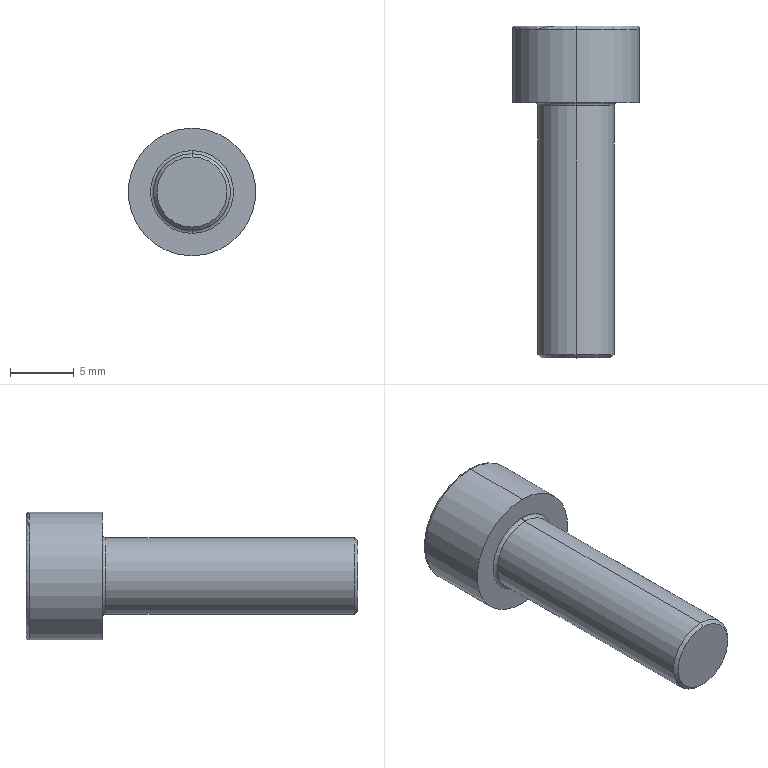Part | STEP file | 1 solid | 20 faces | box 10 x 26 x 10 mm | volume 971.042 mm3 | plane 10 | torus 4 | cylinder 4 | cone 2 | commonest cylinder face diameters 6 x2 10 x2
STEP:
#1=CARTESIAN_POINT('',(0.,-20.,-2.75));
#2=VERTEX_POINT('',#1);
#3=CARTESIAN_POINT('',(0.,-20.,2.75));
#4=VERTEX_POINT('',#3);
#5=CARTESIAN_POINT('',(0.,-20.,0.));
#6=DIRECTION('',(0.,-1.,0.));
#7=DIRECTION('',(0.,0.,-1.));
#8=AXIS2_PLACEMENT_3D('',#5,#6,#7);
#9=CIRCLE('',#8,2.75);
#10=EDGE_CURVE('',#2,#4,#9,.T.);
#11=ORIENTED_EDGE('',*,*,#10,.F.);
#12=CARTESIAN_POINT('',(0.,-19.75,-3.));
#13=VERTEX_POINT('',#12);
#14=CARTESIAN_POINT('',(0.,-20.,-2.75));
#15=DIRECTION('',(0.,0.7071,-0.7071));
#16=VECTOR('',#15,1000.);
#17=LINE('',#14,#16);
#18=EDGE_CURVE('',#2,#13,#17,.T.);
#19=ORIENTED_EDGE('',*,*,#18,.T.);
#20=CARTESIAN_POINT('',(0.,-19.75,3.));
#21=VERTEX_POINT('',#20);
#22=CARTESIAN_POINT('',(0.,-19.75,0.));
#23=DIRECTION('',(0.,1.,0.));
#24=DIRECTION('',(0.,0.,-1.));
#25=AXIS2_PLACEMENT_3D('',#22,#23,#24);
#26=CIRCLE('',#25,3.);
#27=EDGE_CURVE('',#21,#13,#26,.T.);
#28=ORIENTED_EDGE('',*,*,#27,.F.);
#29=CARTESIAN_POINT('',(0.,-20.,2.75));
#30=DIRECTION('',(0.,0.7071,0.7071));
#31=VECTOR('',#30,1000.);
#32=LINE('',#29,#31);
#33=EDGE_CURVE('',#4,#21,#32,.T.);
#34=ORIENTED_EDGE('',*,*,#33,.F.);
#35=EDGE_LOOP('',(#11,#19,#28,#34));
#36=FACE_OUTER_BOUND('',#35,.T.);
#37=CARTESIAN_POINT('',(0.,-20.,0.));
#38=DIRECTION('',(0.,1.,0.));
#39=DIRECTION('',(0.,0.,1.));
#40=AXIS2_PLACEMENT_3D('',#37,#38,#39);
#41=CONICAL_SURFACE('',#40,2.75,0.7854);
#42=ADVANCED_FACE('',(#36),#41,.T.);
#43=CARTESIAN_POINT('',(0.,5.75,-5.));
#44=VERTEX_POINT('',#43);
#45=CARTESIAN_POINT('',(0.,5.75,5.));
#46=VERTEX_POINT('',#45);
#47=CARTESIAN_POINT('',(0.,5.75,0.));
#48=DIRECTION('',(0.,-1.,0.));
#49=DIRECTION('',(0.,0.,1.));
#50=AXIS2_PLACEMENT_3D('',#47,#48,#49);
#51=CIRCLE('',#50,5.);
#52=EDGE_CURVE('',#44,#46,#51,.T.);
#53=ORIENTED_EDGE('',*,*,#52,.F.);
#54=CARTESIAN_POINT('',(0.,6.,-4.75));
#55=VERTEX_POINT('',#54);
#56=CARTESIAN_POINT('',(0.,5.75,-4.75));
#57=DIRECTION('',(1.,0.,0.));
#58=DIRECTION('',(0.,0.,-1.));
#59=AXIS2_PLACEMENT_3D('',#56,#57,#58);
#60=CIRCLE('',#59,0.25);
#61=EDGE_CURVE('',#44,#55,#60,.T.);
#62=ORIENTED_EDGE('',*,*,#61,.T.);
#63=CARTESIAN_POINT('',(0.,6.,4.75));
#64=VERTEX_POINT('',#63);
#65=CARTESIAN_POINT('',(0.,6.,0.));
#66=DIRECTION('',(0.,1.,0.));
#67=DIRECTION('',(0.,0.,1.));
#68=AXIS2_PLACEMENT_3D('',#65,#66,#67);
#69=CIRCLE('',#68,4.75);
#70=EDGE_CURVE('',#64,#55,#69,.T.);
#71=ORIENTED_EDGE('',*,*,#70,.F.);
#72=CARTESIAN_POINT('',(0.,5.75,4.75));
#73=DIRECTION('',(-1.,0.,0.));
#74=DIRECTION('',(0.,0.,1.));
#75=AXIS2_PLACEMENT_3D('',#72,#73,#74);
#76=CIRCLE('',#75,0.25);
#77=EDGE_CURVE('',#46,#64,#76,.T.);
#78=ORIENTED_EDGE('',*,*,#77,.F.);
#79=EDGE_LOOP('',(#53,#62,#71,#78));
#80=FACE_OUTER_BOUND('',#79,.T.);
#81=CARTESIAN_POINT('',(0.,5.75,0.));
#82=DIRECTION('',(0.,1.,0.));
#83=DIRECTION('',(0.,0.,1.));
#84=AXIS2_PLACEMENT_3D('',#81,#82,#83);
#85=TOROIDAL_SURFACE('',#84,4.75,0.25);
#86=ADVANCED_FACE('',(#80),#85,.T.);
#87=CARTESIAN_POINT('',(0.,-0.25,3.));
#88=VERTEX_POINT('',#87);
#89=CARTESIAN_POINT('',(0.,-0.25,-3.));
#90=VERTEX_POINT('',#89);
#91=CARTESIAN_POINT('',(0.,-0.25,0.));
#92=DIRECTION('',(0.,-1.,0.));
#93=DIRECTION('',(0.,0.,-1.));
#94=AXIS2_PLACEMENT_3D('',#91,#92,#93);
#95=CIRCLE('',#94,3.);
#96=EDGE_CURVE('',#88,#90,#95,.T.);
#97=ORIENTED_EDGE('',*,*,#96,.F.);
#98=CARTESIAN_POINT('',(0.,0.,3.25));
#99=VERTEX_POINT('',#98);
#100=CARTESIAN_POINT('',(0.,-0.25,3.25));
#101=DIRECTION('',(1.,0.,0.));
#102=DIRECTION('',(0.,0.,-1.));
#103=AXIS2_PLACEMENT_3D('',#100,#101,#102);
#104=CIRCLE('',#103,0.25);
#105=EDGE_CURVE('',#88,#99,#104,.T.);
#106=ORIENTED_EDGE('',*,*,#105,.T.);
#107=CARTESIAN_POINT('',(0.,0.,-3.25));
#108=VERTEX_POINT('',#107);
#109=CARTESIAN_POINT('',(0.,0.,0.));
#110=DIRECTION('',(0.,1.,0.));
#111=DIRECTION('',(0.,0.,-1.));
#112=AXIS2_PLACEMENT_3D('',#109,#110,#111);
#113=CIRCLE('',#112,3.25);
#114=EDGE_CURVE('',#108,#99,#113,.T.);
#115=ORIENTED_EDGE('',*,*,#114,.F.);
#116=CARTESIAN_POINT('',(0.,-0.25,-3.25));
#117=DIRECTION('',(-1.,0.,0.));
#118=DIRECTION('',(0.,0.,1.));
#119=AXIS2_PLACEMENT_3D('',#116,#117,#118);
#120=CIRCLE('',#119,0.25);
#121=EDGE_CURVE('',#90,#108,#120,.T.);
#122=ORIENTED_EDGE('',*,*,#121,.F.);
#123=EDGE_LOOP('',(#97,#106,#115,#122));
#124=FACE_OUTER_BOUND('',#123,.T.);
#125=CARTESIAN_POINT('',(0.,-0.25,0.));
#126=DIRECTION('',(0.,-1.,0.));
#127=DIRECTION('',(0.,0.,-1.));
#128=AXIS2_PLACEMENT_3D('',#125,#126,#127);
#129=TOROIDAL_SURFACE('',#128,3.25,0.25);
#130=ADVANCED_FACE('',(#124),#129,.F.);
#131=CARTESIAN_POINT('',(0.,-0.25,0.));
#132=DIRECTION('',(0.,-1.,0.));
#133=DIRECTION('',(0.,0.,-1.));
#134=AXIS2_PLACEMENT_3D('',#131,#132,#133);
#135=CIRCLE('',#134,3.);
#136=EDGE_CURVE('',#90,#88,#135,.T.);
#137=ORIENTED_EDGE('',*,*,#136,.T.);
#138=CARTESIAN_POINT('',(0.,0.,3.));
#139=DIRECTION('',(0.,-1.,0.));
#140=VECTOR('',#139,1000.);
#141=LINE('',#138,#140);
#142=EDGE_CURVE('',#88,#21,#141,.T.);
#143=ORIENTED_EDGE('',*,*,#142,.T.);
#144=ORIENTED_EDGE('',*,*,#27,.T.);
#145=CARTESIAN_POINT('',(0.,0.,-3.));
#146=DIRECTION('',(0.,-1.,0.));
#147=VECTOR('',#146,1000.);
#148=LINE('',#145,#147);
#149=EDGE_CURVE('',#90,#13,#148,.T.);
#150=ORIENTED_EDGE('',*,*,#149,.F.);
#151=EDGE_LOOP('',(#137,#143,#144,#150));
#152=FACE_OUTER_BOUND('',#151,.T.);
#153=CARTESIAN_POINT('',(0.,0.,0.));
#154=DIRECTION('',(0.,-1.,0.));
#155=DIRECTION('',(0.,0.,-1.));
#156=AXIS2_PLACEMENT_3D('',#153,#154,#155);
#157=CYLINDRICAL_SURFACE('',#156,3.);
#158=ADVANCED_FACE('',(#152),#157,.T.);
#159=ORIENTED_EDGE('',*,*,#52,.T.);
#160=CARTESIAN_POINT('',(0.,0.,5.));
#161=VERTEX_POINT('',#160);
#162=CARTESIAN_POINT('',(0.,0.,5.));
#163=DIRECTION('',(0.,-1.,0.));
#164=VECTOR('',#163,1000.);
#165=LINE('',#162,#164);
#166=EDGE_CURVE('',#46,#161,#165,.T.);
#167=ORIENTED_EDGE('',*,*,#166,.T.);
#168=CARTESIAN_POINT('',(0.,0.,-5.));
#169=VERTEX_POINT('',#168);
#170=CARTESIAN_POINT('',(0.,0.,0.));
#171=DIRECTION('',(0.,-1.,0.));
#172=DIRECTION('',(0.,0.,-1.));
#173=AXIS2_PLACEMENT_3D('',#170,#171,#172);
#174=CIRCLE('',#173,5.);
#175=EDGE_CURVE('',#169,#161,#174,.T.);
#176=ORIENTED_EDGE('',*,*,#175,.F.);
#177=CARTESIAN_POINT('',(0.,0.,-5.));
#178=DIRECTION('',(0.,-1.,0.));
#179=VECTOR('',#178,1000.);
#180=LINE('',#177,#179);
#181=EDGE_CURVE('',#44,#169,#180,.T.);
#182=ORIENTED_EDGE('',*,*,#181,.F.);
#183=EDGE_LOOP('',(#159,#167,#176,#182));
#184=FACE_OUTER_BOUND('',#183,.T.);
#185=CARTESIAN_POINT('',(0.,0.,0.));
#186=DIRECTION('',(0.,-1.,0.));
#187=DIRECTION('',(0.,0.,-1.));
#188=AXIS2_PLACEMENT_3D('',#185,#186,#187);
#189=CYLINDRICAL_SURFACE('',#188,5.);
#190=ADVANCED_FACE('',(#184),#189,.T.);
#191=ORIENTED_EDGE('',*,*,#70,.T.);
#192=CARTESIAN_POINT('',(0.,6.,0.));
#193=DIRECTION('',(0.,1.,0.));
#194=DIRECTION('',(0.,0.,1.));
#195=AXIS2_PLACEMENT_3D('',#192,#193,#194);
#196=CIRCLE('',#195,4.75);
#197=EDGE_CURVE('',#55,#64,#196,.T.);
#198=ORIENTED_EDGE('',*,*,#197,.T.);
#199=EDGE_LOOP('',(#191,#198));
#200=FACE_OUTER_BOUND('',#199,.T.);
#201=CARTESIAN_POINT('',(0.,6.,-2.887));
#202=VERTEX_POINT('',#201);
#203=CARTESIAN_POINT('',(-2.5,6.,-1.443));
#204=VERTEX_POINT('',#203);
#205=CARTESIAN_POINT('',(0.,6.,-2.887));
#206=DIRECTION('',(-0.866,0.,0.5));
#207=VECTOR('',#206,1000.);
#208=LINE('',#205,#207);
#209=EDGE_CURVE('',#202,#204,#208,.T.);
#210=ORIENTED_EDGE('',*,*,#209,.F.);
#211=CARTESIAN_POINT('',(2.5,6.,-1.443));
#212=VERTEX_POINT('',#211);
#213=CARTESIAN_POINT('',(2.5,6.,-1.443));
#214=DIRECTION('',(-0.866,0.,-0.5));
#215=VECTOR('',#214,1000.);
#216=LINE('',#213,#215);
#217=EDGE_CURVE('',#212,#202,#216,.T.);
#218=ORIENTED_EDGE('',*,*,#217,.F.);
#219=CARTESIAN_POINT('',(2.5,6.,1.443));
#220=VERTEX_POINT('',#219);
#221=CARTESIAN_POINT('',(2.5,6.,1.443));
#222=DIRECTION('',(0.,0.,-1.));
#223=VECTOR('',#222,1000.);
#224=LINE('',#221,#223);
#225=EDGE_CURVE('',#220,#212,#224,.T.);
#226=ORIENTED_EDGE('',*,*,#225,.F.);
#227=CARTESIAN_POINT('',(0.,6.,2.887));
#228=VERTEX_POINT('',#227);
#229=CARTESIAN_POINT('',(0.,6.,2.887));
#230=DIRECTION('',(0.866,0.,-0.5));
#231=VECTOR('',#230,1000.);
#232=LINE('',#229,#231);
#233=EDGE_CURVE('',#228,#220,#232,.T.);
#234=ORIENTED_EDGE('',*,*,#233,.F.);
#235=CARTESIAN_POINT('',(-2.5,6.,1.443));
#236=VERTEX_POINT('',#235);
#237=CARTESIAN_POINT('',(-2.5,6.,1.443));
#238=DIRECTION('',(0.866,0.,0.5));
#239=VECTOR('',#238,1000.);
#240=LINE('',#237,#239);
#241=EDGE_CURVE('',#236,#228,#240,.T.);
#242=ORIENTED_EDGE('',*,*,#241,.F.);
#243=CARTESIAN_POINT('',(-2.5,6.,-1.443));
#244=DIRECTION('',(0.,0.,1.));
#245=VECTOR('',#244,1000.);
#246=LINE('',#243,#245);
#247=EDGE_CURVE('',#204,#236,#246,.T.);
#248=ORIENTED_EDGE('',*,*,#247,.F.);
#249=EDGE_LOOP('',(#210,#218,#226,#234,#242,#248));
#250=FACE_BOUND('',#249,.T.);
#251=CARTESIAN_POINT('',(0.,6.,0.));
#252=DIRECTION('',(0.,1.,0.));
#253=DIRECTION('',(0.,0.,1.));
#254=AXIS2_PLACEMENT_3D('',#251,#252,#253);
#255=PLANE('',#254);
#256=ADVANCED_FACE('',(#200,#250),#255,.T.);
#257=ORIENTED_EDGE('',*,*,#166,.F.);
#258=CARTESIAN_POINT('',(0.,5.75,0.));
#259=DIRECTION('',(0.,-1.,0.));
#260=DIRECTION('',(0.,0.,1.));
#261=AXIS2_PLACEMENT_3D('',#258,#259,#260);
#262=CIRCLE('',#261,5.);
#263=EDGE_CURVE('',#46,#44,#262,.T.);
#264=ORIENTED_EDGE('',*,*,#263,.T.);
#265=ORIENTED_EDGE('',*,*,#181,.T.);
#266=CARTESIAN_POINT('',(0.,0.,0.));
#267=DIRECTION('',(0.,-1.,0.));
#268=DIRECTION('',(0.,0.,-1.));
#269=AXIS2_PLACEMENT_3D('',#266,#267,#268);
#270=CIRCLE('',#269,5.);
#271=EDGE_CURVE('',#161,#169,#270,.T.);
#272=ORIENTED_EDGE('',*,*,#271,.F.);
#273=EDGE_LOOP('',(#257,#264,#265,#272));
#274=FACE_OUTER_BOUND('',#273,.T.);
#275=CARTESIAN_POINT('',(0.,0.,0.));
#276=DIRECTION('',(0.,-1.,0.));
#277=DIRECTION('',(0.,0.,-1.));
#278=AXIS2_PLACEMENT_3D('',#275,#276,#277);
#279=CYLINDRICAL_SURFACE('',#278,5.);
#280=ADVANCED_FACE('',(#274),#279,.T.);
#281=ORIENTED_EDGE('',*,*,#114,.T.);
#282=CARTESIAN_POINT('',(0.,0.,0.));
#283=DIRECTION('',(0.,1.,0.));
#284=DIRECTION('',(0.,0.,-1.));
#285=AXIS2_PLACEMENT_3D('',#282,#283,#284);
#286=CIRCLE('',#285,3.25);
#287=EDGE_CURVE('',#99,#108,#286,.T.);
#288=ORIENTED_EDGE('',*,*,#287,.T.);
#289=EDGE_LOOP('',(#281,#288));
#290=FACE_BOUND('',#289,.T.);
#291=ORIENTED_EDGE('',*,*,#175,.T.);
#292=ORIENTED_EDGE('',*,*,#271,.T.);
#293=EDGE_LOOP('',(#291,#292));
#294=FACE_OUTER_BOUND('',#293,.T.);
#295=CARTESIAN_POINT('',(5.,0.,0.));
#296=DIRECTION('',(0.,-1.,0.));
#297=DIRECTION('',(0.,0.,-1.));
#298=AXIS2_PLACEMENT_3D('',#295,#296,#297);
#299=PLANE('',#298);
#300=ADVANCED_FACE('',(#290,#294),#299,.T.);
#301=ORIENTED_EDGE('',*,*,#142,.F.);
#302=ORIENTED_EDGE('',*,*,#96,.T.);
#303=ORIENTED_EDGE('',*,*,#149,.T.);
#304=CARTESIAN_POINT('',(0.,-19.75,0.));
#305=DIRECTION('',(0.,1.,0.));
#306=DIRECTION('',(0.,0.,-1.));
#307=AXIS2_PLACEMENT_3D('',#304,#305,#306);
#308=CIRCLE('',#307,3.);
#309=EDGE_CURVE('',#13,#21,#308,.T.);
#310=ORIENTED_EDGE('',*,*,#309,.T.);
#311=EDGE_LOOP('',(#301,#302,#303,#310));
#312=FACE_OUTER_BOUND('',#311,.T.);
#313=CARTESIAN_POINT('',(0.,0.,0.));
#314=DIRECTION('',(0.,-1.,0.));
#315=DIRECTION('',(0.,0.,-1.));
#316=AXIS2_PLACEMENT_3D('',#313,#314,#315);
#317=CYLINDRICAL_SURFACE('',#316,3.);
#318=ADVANCED_FACE('',(#312),#317,.T.);
#319=CARTESIAN_POINT('',(0.,-20.,0.));
#320=DIRECTION('',(0.,-1.,0.));
#321=DIRECTION('',(0.,0.,-1.));
#322=AXIS2_PLACEMENT_3D('',#319,#320,#321);
#323=CIRCLE('',#322,2.75);
#324=EDGE_CURVE('',#4,#2,#323,.T.);
#325=ORIENTED_EDGE('',*,*,#324,.T.);
#326=ORIENTED_EDGE('',*,*,#10,.T.);
#327=EDGE_LOOP('',(#325,#326));
#328=FACE_OUTER_BOUND('',#327,.T.);
#329=CARTESIAN_POINT('',(3.,-20.,0.));
#330=DIRECTION('',(0.,-1.,0.));
#331=DIRECTION('',(0.,0.,-1.));
#332=AXIS2_PLACEMENT_3D('',#329,#330,#331);
#333=PLANE('',#332);
#334=ADVANCED_FACE('',(#328),#333,.T.);
#335=ORIENTED_EDGE('',*,*,#209,.T.);
#336=CARTESIAN_POINT('',(-2.5,3.,-1.443));
#337=VERTEX_POINT('',#336);
#338=CARTESIAN_POINT('',(-2.5,3.,-1.443));
#339=DIRECTION('',(0.,1.,0.));
#340=VECTOR('',#339,1000.);
#341=LINE('',#338,#340);
#342=EDGE_CURVE('',#337,#204,#341,.T.);
#343=ORIENTED_EDGE('',*,*,#342,.F.);
#344=CARTESIAN_POINT('',(0.,3.,-2.887));
#345=VERTEX_POINT('',#344);
#346=CARTESIAN_POINT('',(0.,3.,-2.887));
#347=DIRECTION('',(-0.866,0.,0.5));
#348=VECTOR('',#347,1000.);
#349=LINE('',#346,#348);
#350=EDGE_CURVE('',#345,#337,#349,.T.);
#351=ORIENTED_EDGE('',*,*,#350,.F.);
#352=CARTESIAN_POINT('',(0.,3.,-2.887));
#353=DIRECTION('',(0.,1.,0.));
#354=VECTOR('',#353,1000.);
#355=LINE('',#352,#354);
#356=EDGE_CURVE('',#345,#202,#355,.T.);
#357=ORIENTED_EDGE('',*,*,#356,.T.);
#358=EDGE_LOOP('',(#335,#343,#351,#357));
#359=FACE_OUTER_BOUND('',#358,.T.);
#360=CARTESIAN_POINT('',(0.,3.,-2.887));
#361=DIRECTION('',(-0.5,0.,-0.866));
#362=DIRECTION('',(-0.866,0.,0.5));
#363=AXIS2_PLACEMENT_3D('',#360,#361,#362);
#364=PLANE('',#363);
#365=ADVANCED_FACE('',(#359),#364,.F.);
#366=ORIENTED_EDGE('',*,*,#217,.T.);
#367=ORIENTED_EDGE('',*,*,#356,.F.);
#368=CARTESIAN_POINT('',(2.5,3.,-1.443));
#369=VERTEX_POINT('',#368);
#370=CARTESIAN_POINT('',(2.5,3.,-1.443));
#371=DIRECTION('',(-0.866,0.,-0.5));
#372=VECTOR('',#371,1000.);
#373=LINE('',#370,#372);
#374=EDGE_CURVE('',#369,#345,#373,.T.);
#375=ORIENTED_EDGE('',*,*,#374,.F.);
#376=CARTESIAN_POINT('',(2.5,3.,-1.443));
#377=DIRECTION('',(0.,1.,0.));
#378=VECTOR('',#377,1000.);
#379=LINE('',#376,#378);
#380=EDGE_CURVE('',#369,#212,#379,.T.);
#381=ORIENTED_EDGE('',*,*,#380,.T.);
#382=EDGE_LOOP('',(#366,#367,#375,#381));
#383=FACE_OUTER_BOUND('',#382,.T.);
#384=CARTESIAN_POINT('',(2.5,3.,-1.443));
#385=DIRECTION('',(0.5,0.,-0.866));
#386=DIRECTION('',(-0.866,0.,-0.5));
#387=AXIS2_PLACEMENT_3D('',#384,#385,#386);
#388=PLANE('',#387);
#389=ADVANCED_FACE('',(#383),#388,.F.);
#390=ORIENTED_EDGE('',*,*,#225,.T.);
#391=ORIENTED_EDGE('',*,*,#380,.F.);
#392=CARTESIAN_POINT('',(2.5,3.,1.443));
#393=VERTEX_POINT('',#392);
#394=CARTESIAN_POINT('',(2.5,3.,1.443));
#395=DIRECTION('',(0.,0.,-1.));
#396=VECTOR('',#395,1000.);
#397=LINE('',#394,#396);
#398=EDGE_CURVE('',#393,#369,#397,.T.);
#399=ORIENTED_EDGE('',*,*,#398,.F.);
#400=CARTESIAN_POINT('',(2.5,3.,1.443));
#401=DIRECTION('',(0.,1.,0.));
#402=VECTOR('',#401,1000.);
#403=LINE('',#400,#402);
#404=EDGE_CURVE('',#393,#220,#403,.T.);
#405=ORIENTED_EDGE('',*,*,#404,.T.);
#406=EDGE_LOOP('',(#390,#391,#399,#405));
#407=FACE_OUTER_BOUND('',#406,.T.);
#408=CARTESIAN_POINT('',(2.5,3.,1.443));
#409=DIRECTION('',(1.,0.,0.));
#410=DIRECTION('',(0.,0.,-1.));
#411=AXIS2_PLACEMENT_3D('',#408,#409,#410);
#412=PLANE('',#411);
#413=ADVANCED_FACE('',(#407),#412,.F.);
#414=ORIENTED_EDGE('',*,*,#233,.T.);
#415=ORIENTED_EDGE('',*,*,#404,.F.);
#416=CARTESIAN_POINT('',(0.,3.,2.887));
#417=VERTEX_POINT('',#416);
#418=CARTESIAN_POINT('',(0.,3.,2.887));
#419=DIRECTION('',(0.866,0.,-0.5));
#420=VECTOR('',#419,1000.);
#421=LINE('',#418,#420);
#422=EDGE_CURVE('',#417,#393,#421,.T.);
#423=ORIENTED_EDGE('',*,*,#422,.F.);
#424=CARTESIAN_POINT('',(0.,3.,2.887));
#425=DIRECTION('',(0.,1.,0.));
#426=VECTOR('',#425,1000.);
#427=LINE('',#424,#426);
#428=EDGE_CURVE('',#417,#228,#427,.T.);
#429=ORIENTED_EDGE('',*,*,#428,.T.);
#430=EDGE_LOOP('',(#414,#415,#423,#429));
#431=FACE_OUTER_BOUND('',#430,.T.);
#432=CARTESIAN_POINT('',(0.,3.,2.887));
#433=DIRECTION('',(0.5,0.,0.866));
#434=DIRECTION('',(0.866,0.,-0.5));
#435=AXIS2_PLACEMENT_3D('',#432,#433,#434);
#436=PLANE('',#435);
#437=ADVANCED_FACE('',(#431),#436,.F.);
#438=ORIENTED_EDGE('',*,*,#241,.T.);
#439=ORIENTED_EDGE('',*,*,#428,.F.);
#440=CARTESIAN_POINT('',(-2.5,3.,1.443));
#441=VERTEX_POINT('',#440);
#442=CARTESIAN_POINT('',(-2.5,3.,1.443));
#443=DIRECTION('',(0.866,0.,0.5));
#444=VECTOR('',#443,1000.);
#445=LINE('',#442,#444);
#446=EDGE_CURVE('',#441,#417,#445,.T.);
#447=ORIENTED_EDGE('',*,*,#446,.F.);
#448=CARTESIAN_POINT('',(-2.5,3.,1.443));
#449=DIRECTION('',(0.,1.,0.));
#450=VECTOR('',#449,1000.);
#451=LINE('',#448,#450);
#452=EDGE_CURVE('',#441,#236,#451,.T.);
#453=ORIENTED_EDGE('',*,*,#452,.T.);
#454=EDGE_LOOP('',(#438,#439,#447,#453));
#455=FACE_OUTER_BOUND('',#454,.T.);
#456=CARTESIAN_POINT('',(-2.5,3.,1.443));
#457=DIRECTION('',(-0.5,0.,0.866));
#458=DIRECTION('',(0.866,0.,0.5));
#459=AXIS2_PLACEMENT_3D('',#456,#457,#458);
#460=PLANE('',#459);
#461=ADVANCED_FACE('',(#455),#460,.F.);
#462=ORIENTED_EDGE('',*,*,#247,.T.);
#463=ORIENTED_EDGE('',*,*,#452,.F.);
#464=CARTESIAN_POINT('',(-2.5,3.,-1.443));
#465=DIRECTION('',(0.,0.,1.));
#466=VECTOR('',#465,1000.);
#467=LINE('',#464,#466);
#468=EDGE_CURVE('',#337,#441,#467,.T.);
#469=ORIENTED_EDGE('',*,*,#468,.F.);
#470=ORIENTED_EDGE('',*,*,#342,.T.);
#471=EDGE_LOOP('',(#462,#463,#469,#470));
#472=FACE_OUTER_BOUND('',#471,.T.);
#473=CARTESIAN_POINT('',(-2.5,3.,-1.443));
#474=DIRECTION('',(-1.,0.,0.));
#475=DIRECTION('',(0.,0.,1.));
#476=AXIS2_PLACEMENT_3D('',#473,#474,#475);
#477=PLANE('',#476);
#478=ADVANCED_FACE('',(#472),#477,.F.);
#479=ORIENTED_EDGE('',*,*,#350,.T.);
#480=ORIENTED_EDGE('',*,*,#468,.T.);
#481=ORIENTED_EDGE('',*,*,#446,.T.);
#482=ORIENTED_EDGE('',*,*,#422,.T.);
#483=ORIENTED_EDGE('',*,*,#398,.T.);
#484=ORIENTED_EDGE('',*,*,#374,.T.);
#485=EDGE_LOOP('',(#479,#480,#481,#482,#483,#484));
#486=FACE_OUTER_BOUND('',#485,.T.);
#487=CARTESIAN_POINT('',(0.,3.,0.));
#488=DIRECTION('',(0.,1.,0.));
#489=DIRECTION('',(0.,0.,1.));
#490=AXIS2_PLACEMENT_3D('',#487,#488,#489);
#491=PLANE('',#490);
#492=ADVANCED_FACE('',(#486),#491,.T.);
#493=ORIENTED_EDGE('',*,*,#105,.F.);
#494=ORIENTED_EDGE('',*,*,#136,.F.);
#495=ORIENTED_EDGE('',*,*,#121,.T.);
#496=ORIENTED_EDGE('',*,*,#287,.F.);
#497=EDGE_LOOP('',(#493,#494,#495,#496));
#498=FACE_OUTER_BOUND('',#497,.T.);
#499=CARTESIAN_POINT('',(0.,-0.25,0.));
#500=DIRECTION('',(0.,-1.,0.));
#501=DIRECTION('',(0.,0.,-1.));
#502=AXIS2_PLACEMENT_3D('',#499,#500,#501);
#503=TOROIDAL_SURFACE('',#502,3.25,0.25);
#504=ADVANCED_FACE('',(#498),#503,.F.);
#505=ORIENTED_EDGE('',*,*,#61,.F.);
#506=ORIENTED_EDGE('',*,*,#263,.F.);
#507=ORIENTED_EDGE('',*,*,#77,.T.);
#508=ORIENTED_EDGE('',*,*,#197,.F.);
#509=EDGE_LOOP('',(#505,#506,#507,#508));
#510=FACE_OUTER_BOUND('',#509,.T.);
#511=CARTESIAN_POINT('',(0.,5.75,0.));
#512=DIRECTION('',(0.,1.,0.));
#513=DIRECTION('',(0.,0.,1.));
#514=AXIS2_PLACEMENT_3D('',#511,#512,#513);
#515=TOROIDAL_SURFACE('',#514,4.75,0.25);
#516=ADVANCED_FACE('',(#510),#515,.T.);
#517=ORIENTED_EDGE('',*,*,#18,.F.);
#518=ORIENTED_EDGE('',*,*,#324,.F.);
#519=ORIENTED_EDGE('',*,*,#33,.T.);
#520=ORIENTED_EDGE('',*,*,#309,.F.);
#521=EDGE_LOOP('',(#517,#518,#519,#520));
#522=FACE_OUTER_BOUND('',#521,.T.);
#523=CARTESIAN_POINT('',(0.,-20.,0.));
#524=DIRECTION('',(0.,1.,0.));
#525=DIRECTION('',(0.,0.,1.));
#526=AXIS2_PLACEMENT_3D('',#523,#524,#525);
#527=CONICAL_SURFACE('',#526,2.75,0.7854);
#528=ADVANCED_FACE('',(#522),#527,.T.);
#529=CLOSED_SHELL('',(#42,#86,#130,#158,#190,#256,#280,#300,#318,#334,#365,#389,#413,#437,#461,#478,#492,#504,#516,#528));
#530=MANIFOLD_SOLID_BREP('',#529);
#531=CARTESIAN_POINT('',(0.,0.,0.));
#532=DIRECTION('',(0.,0.,1.));
#533=DIRECTION('',(1.,0.,0.));
#534=AXIS2_PLACEMENT_3D('',#531,#532,#533);
#535=(LENGTH_UNIT()NAMED_UNIT(*)SI_UNIT(.MILLI.,.METRE.));
#536=UNCERTAINTY_MEASURE_WITH_UNIT(LENGTH_MEASURE(0.00001),#535,'','');
#537=(NAMED_UNIT(*)PLANE_ANGLE_UNIT()SI_UNIT($,.RADIAN.));
#538=(NAMED_UNIT(*)SI_UNIT($,.STERADIAN.)SOLID_ANGLE_UNIT());
#539=(GEOMETRIC_REPRESENTATION_CONTEXT(3)GLOBAL_UNCERTAINTY_ASSIGNED_CONTEXT((#536))GLOBAL_UNIT_ASSIGNED_CONTEXT((#535,#537,#538))REPRESENTATION_CONTEXT('',''));
#540=ADVANCED_BREP_SHAPE_REPRESENTATION('',(#530,#534),#539);